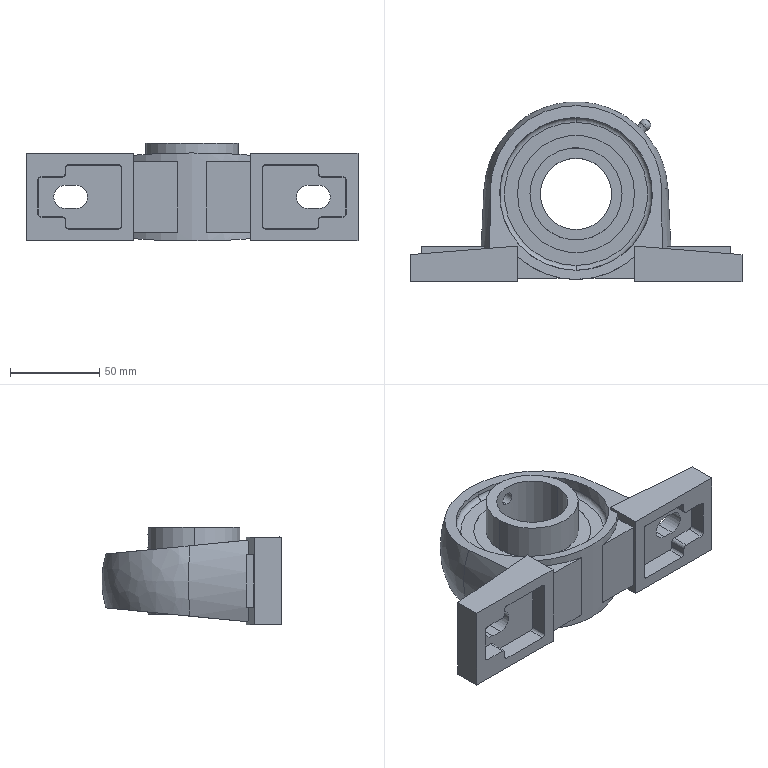Part | SolidWorks | features Revolution 5, Boss 3, Cut 3, RevCut 2, CirPattern 1, Extrusion 1, SweepCut 1 | 1 solid | 123 faces | box 186 x 100.8 x 54.842 mm | volume 267001 mm3 | plane 61 | cylinder 27 | cone 16 | sphere 8 | torus 8 | spline 3 | commonest cylinder face diameters 51.6 x6 65.64 x6 85.524 x6 13 x4 7.134 x2 40 x2